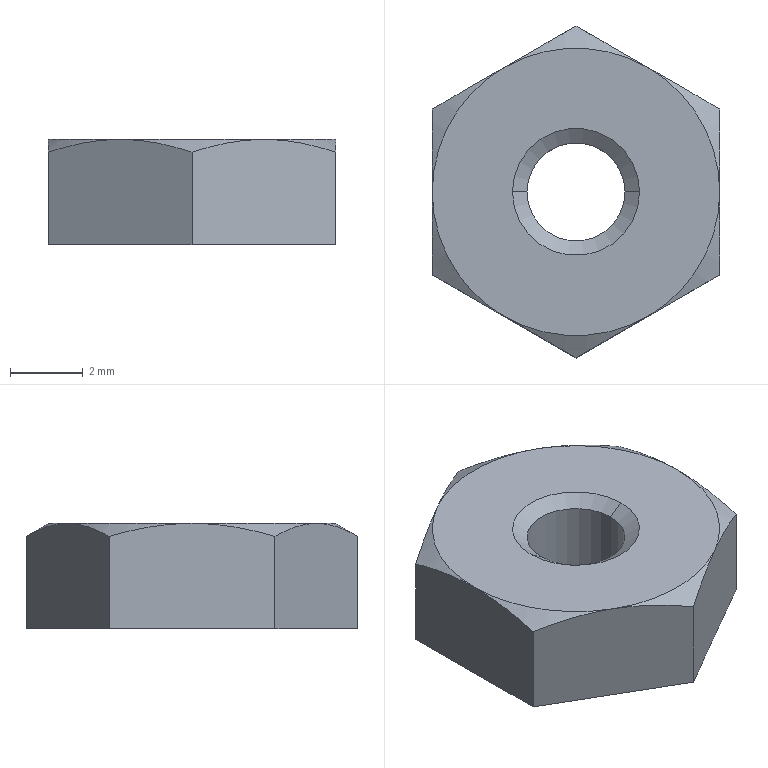Part | SolidWorks | features BaseBody 1 | 1 solid | 22 faces | box 7.925 x 9.151 x 2.896 mm | volume 139.153 mm3 | cone 10 | plane 8 | cylinder 4 | commonest cylinder face diameters 2.705 x2 3.505 x2
STEP:
#1=CARTESIAN_POINT('',(1.753,0.,-2.896));
#2=VERTEX_POINT('',#1);
#3=CARTESIAN_POINT('',(-1.753,0.,-2.896));
#4=VERTEX_POINT('',#3);
#5=CARTESIAN_POINT('',(0.,0.,-2.896));
#6=DIRECTION('',(0.,0.,-1.));
#7=DIRECTION('',(1.,0.,0.));
#8=AXIS2_PLACEMENT_3D('',#5,#6,#7);
#9=CIRCLE('',#8,1.753);
#10=EDGE_CURVE('',#2,#4,#9,.T.);
#11=ORIENTED_EDGE('',*,*,#10,.T.);
#12=CARTESIAN_POINT('',(-1.753,0.,-2.87));
#13=VERTEX_POINT('',#12);
#14=CARTESIAN_POINT('',(-1.753,0.,-2.896));
#15=DIRECTION('',(0.,0.,1.));
#16=VECTOR('',#15,1000.);
#17=LINE('',#14,#16);
#18=EDGE_CURVE('',#4,#13,#17,.T.);
#19=ORIENTED_EDGE('',*,*,#18,.T.);
#20=CARTESIAN_POINT('',(1.753,0.,-2.87));
#21=VERTEX_POINT('',#20);
#22=CARTESIAN_POINT('',(0.,0.,-2.87));
#23=DIRECTION('',(0.,0.,1.));
#24=DIRECTION('',(1.,0.,0.));
#25=AXIS2_PLACEMENT_3D('',#22,#23,#24);
#26=CIRCLE('',#25,1.753);
#27=EDGE_CURVE('',#13,#21,#26,.T.);
#28=ORIENTED_EDGE('',*,*,#27,.T.);
#29=CARTESIAN_POINT('',(1.753,0.,-2.896));
#30=DIRECTION('',(0.,0.,1.));
#31=VECTOR('',#30,1000.);
#32=LINE('',#29,#31);
#33=EDGE_CURVE('',#2,#21,#32,.T.);
#34=ORIENTED_EDGE('',*,*,#33,.F.);
#35=EDGE_LOOP('',(#11,#19,#28,#34));
#36=FACE_OUTER_BOUND('',#35,.T.);
#37=CARTESIAN_POINT('',(0.,0.,-2.896));
#38=DIRECTION('',(0.,0.,1.));
#39=DIRECTION('',(1.,0.,0.));
#40=AXIS2_PLACEMENT_3D('',#37,#38,#39);
#41=CYLINDRICAL_SURFACE('',#40,1.753);
#42=ADVANCED_FACE('',(#36),#41,.F.);
#43=CARTESIAN_POINT('',(-1.353,0.,-2.59));
#44=VERTEX_POINT('',#43);
#45=CARTESIAN_POINT('',(1.353,0.,-2.59));
#46=VERTEX_POINT('',#45);
#47=CARTESIAN_POINT('',(0.,0.,-2.59));
#48=DIRECTION('',(0.,0.,1.));
#49=DIRECTION('',(-1.,0.,0.));
#50=AXIS2_PLACEMENT_3D('',#47,#48,#49);
#51=CIRCLE('',#50,1.353);
#52=EDGE_CURVE('',#44,#46,#51,.T.);
#53=ORIENTED_EDGE('',*,*,#52,.T.);
#54=CARTESIAN_POINT('',(1.353,0.,-2.59));
#55=DIRECTION('',(0.8192,0.,-0.5736));
#56=VECTOR('',#55,1000.);
#57=LINE('',#54,#56);
#58=EDGE_CURVE('',#46,#21,#57,.T.);
#59=ORIENTED_EDGE('',*,*,#58,.T.);
#60=ORIENTED_EDGE('',*,*,#27,.F.);
#61=CARTESIAN_POINT('',(-1.353,0.,-2.59));
#62=DIRECTION('',(-0.8192,0.,-0.5736));
#63=VECTOR('',#62,1000.);
#64=LINE('',#61,#63);
#65=EDGE_CURVE('',#44,#13,#64,.T.);
#66=ORIENTED_EDGE('',*,*,#65,.F.);
#67=EDGE_LOOP('',(#53,#59,#60,#66));
#68=FACE_OUTER_BOUND('',#67,.T.);
#69=CARTESIAN_POINT('',(0.,0.,-2.59));
#70=DIRECTION('',(0.,0.,-1.));
#71=DIRECTION('',(-1.,0.,0.));
#72=AXIS2_PLACEMENT_3D('',#69,#70,#71);
#73=CONICAL_SURFACE('',#72,1.353,0.9599);
#74=ADVANCED_FACE('',(#68),#73,.F.);
#75=ORIENTED_EDGE('',*,*,#52,.F.);
#76=CARTESIAN_POINT('',(-1.353,0.,-0.2801));
#77=VERTEX_POINT('',#76);
#78=CARTESIAN_POINT('',(-1.353,0.,-2.59));
#79=DIRECTION('',(0.,0.,1.));
#80=VECTOR('',#79,1000.);
#81=LINE('',#78,#80);
#82=EDGE_CURVE('',#44,#77,#81,.T.);
#83=ORIENTED_EDGE('',*,*,#82,.T.);
#84=CARTESIAN_POINT('',(1.353,0.,-0.2801));
#85=VERTEX_POINT('',#84);
#86=CARTESIAN_POINT('',(0.,0.,-0.2801));
#87=DIRECTION('',(0.,0.,1.));
#88=DIRECTION('',(1.,0.,0.));
#89=AXIS2_PLACEMENT_3D('',#86,#87,#88);
#90=CIRCLE('',#89,1.353);
#91=EDGE_CURVE('',#77,#85,#90,.T.);
#92=ORIENTED_EDGE('',*,*,#91,.T.);
#93=CARTESIAN_POINT('',(1.353,0.,-2.59));
#94=DIRECTION('',(0.,0.,1.));
#95=VECTOR('',#94,1000.);
#96=LINE('',#93,#95);
#97=EDGE_CURVE('',#46,#85,#96,.T.);
#98=ORIENTED_EDGE('',*,*,#97,.F.);
#99=EDGE_LOOP('',(#75,#83,#92,#98));
#100=FACE_OUTER_BOUND('',#99,.T.);
#101=CARTESIAN_POINT('',(0.,0.,-2.59));
#102=DIRECTION('',(0.,0.,1.));
#103=DIRECTION('',(1.,0.,0.));
#104=AXIS2_PLACEMENT_3D('',#101,#102,#103);
#105=CYLINDRICAL_SURFACE('',#104,1.353);
#106=ADVANCED_FACE('',(#100),#105,.F.);
#107=ORIENTED_EDGE('',*,*,#91,.F.);
#108=CARTESIAN_POINT('',(-1.753,0.,0.));
#109=VERTEX_POINT('',#108);
#110=CARTESIAN_POINT('',(-1.353,0.,-0.2801));
#111=DIRECTION('',(-0.8192,0.,0.5736));
#112=VECTOR('',#111,1000.);
#113=LINE('',#110,#112);
#114=EDGE_CURVE('',#77,#109,#113,.T.);
#115=ORIENTED_EDGE('',*,*,#114,.T.);
#116=CARTESIAN_POINT('',(1.753,0.,0.));
#117=VERTEX_POINT('',#116);
#118=CARTESIAN_POINT('',(0.,0.,0.));
#119=DIRECTION('',(0.,0.,1.));
#120=DIRECTION('',(1.,0.,0.));
#121=AXIS2_PLACEMENT_3D('',#118,#119,#120);
#122=CIRCLE('',#121,1.753);
#123=EDGE_CURVE('',#109,#117,#122,.T.);
#124=ORIENTED_EDGE('',*,*,#123,.T.);
#125=CARTESIAN_POINT('',(1.353,0.,-0.2801));
#126=DIRECTION('',(0.8192,0.,0.5736));
#127=VECTOR('',#126,1000.);
#128=LINE('',#125,#127);
#129=EDGE_CURVE('',#85,#117,#128,.T.);
#130=ORIENTED_EDGE('',*,*,#129,.F.);
#131=EDGE_LOOP('',(#107,#115,#124,#130));
#132=FACE_OUTER_BOUND('',#131,.T.);
#133=CARTESIAN_POINT('',(0.,0.,-0.2801));
#134=DIRECTION('',(0.,0.,1.));
#135=DIRECTION('',(1.,0.,0.));
#136=AXIS2_PLACEMENT_3D('',#133,#134,#135);
#137=CONICAL_SURFACE('',#136,1.353,0.9599);
#138=ADVANCED_FACE('',(#132),#137,.F.);
#139=ORIENTED_EDGE('',*,*,#18,.F.);
#140=CARTESIAN_POINT('',(0.,0.,-2.896));
#141=DIRECTION('',(0.,0.,-1.));
#142=DIRECTION('',(1.,0.,0.));
#143=AXIS2_PLACEMENT_3D('',#140,#141,#142);
#144=CIRCLE('',#143,1.753);
#145=EDGE_CURVE('',#4,#2,#144,.T.);
#146=ORIENTED_EDGE('',*,*,#145,.T.);
#147=ORIENTED_EDGE('',*,*,#33,.T.);
#148=CARTESIAN_POINT('',(0.,0.,-2.87));
#149=DIRECTION('',(0.,0.,1.));
#150=DIRECTION('',(1.,0.,0.));
#151=AXIS2_PLACEMENT_3D('',#148,#149,#150);
#152=CIRCLE('',#151,1.753);
#153=EDGE_CURVE('',#21,#13,#152,.T.);
#154=ORIENTED_EDGE('',*,*,#153,.T.);
#155=EDGE_LOOP('',(#139,#146,#147,#154));
#156=FACE_OUTER_BOUND('',#155,.T.);
#157=CARTESIAN_POINT('',(0.,0.,-2.896));
#158=DIRECTION('',(0.,0.,1.));
#159=DIRECTION('',(1.,0.,0.));
#160=AXIS2_PLACEMENT_3D('',#157,#158,#159);
#161=CYLINDRICAL_SURFACE('',#160,1.753);
#162=ADVANCED_FACE('',(#156),#161,.F.);
#163=ORIENTED_EDGE('',*,*,#58,.F.);
#164=CARTESIAN_POINT('',(0.,0.,-2.59));
#165=DIRECTION('',(0.,0.,1.));
#166=DIRECTION('',(-1.,0.,0.));
#167=AXIS2_PLACEMENT_3D('',#164,#165,#166);
#168=CIRCLE('',#167,1.353);
#169=EDGE_CURVE('',#46,#44,#168,.T.);
#170=ORIENTED_EDGE('',*,*,#169,.T.);
#171=ORIENTED_EDGE('',*,*,#65,.T.);
#172=ORIENTED_EDGE('',*,*,#153,.F.);
#173=EDGE_LOOP('',(#163,#170,#171,#172));
#174=FACE_OUTER_BOUND('',#173,.T.);
#175=CARTESIAN_POINT('',(0.,0.,-2.59));
#176=DIRECTION('',(0.,0.,-1.));
#177=DIRECTION('',(-1.,0.,0.));
#178=AXIS2_PLACEMENT_3D('',#175,#176,#177);
#179=CONICAL_SURFACE('',#178,1.353,0.9599);
#180=ADVANCED_FACE('',(#174),#179,.F.);
#181=ORIENTED_EDGE('',*,*,#10,.F.);
#182=ORIENTED_EDGE('',*,*,#145,.F.);
#183=EDGE_LOOP('',(#181,#182));
#184=FACE_BOUND('',#183,.T.);
#185=CARTESIAN_POINT('',(0.,-4.575,-2.896));
#186=VERTEX_POINT('',#185);
#187=CARTESIAN_POINT('',(-3.962,-2.288,-2.896));
#188=VERTEX_POINT('',#187);
#189=CARTESIAN_POINT('',(0.,-4.575,-2.896));
#190=DIRECTION('',(-0.866,0.5,0.));
#191=VECTOR('',#190,1000.);
#192=LINE('',#189,#191);
#193=EDGE_CURVE('',#186,#188,#192,.T.);
#194=ORIENTED_EDGE('',*,*,#193,.T.);
#195=CARTESIAN_POINT('',(-3.962,2.288,-2.896));
#196=VERTEX_POINT('',#195);
#197=CARTESIAN_POINT('',(-3.962,0.,-2.896));
#198=DIRECTION('',(0.,1.,0.));
#199=VECTOR('',#198,1000.);
#200=LINE('',#197,#199);
#201=EDGE_CURVE('',#188,#196,#200,.T.);
#202=ORIENTED_EDGE('',*,*,#201,.T.);
#203=CARTESIAN_POINT('',(0.,4.575,-2.896));
#204=VERTEX_POINT('',#203);
#205=CARTESIAN_POINT('',(-3.962,2.288,-2.896));
#206=DIRECTION('',(0.866,0.5,0.));
#207=VECTOR('',#206,1000.);
#208=LINE('',#205,#207);
#209=EDGE_CURVE('',#196,#204,#208,.T.);
#210=ORIENTED_EDGE('',*,*,#209,.T.);
#211=CARTESIAN_POINT('',(3.962,2.288,-2.896));
#212=VERTEX_POINT('',#211);
#213=CARTESIAN_POINT('',(0.,4.575,-2.896));
#214=DIRECTION('',(0.866,-0.5,0.));
#215=VECTOR('',#214,1000.);
#216=LINE('',#213,#215);
#217=EDGE_CURVE('',#204,#212,#216,.T.);
#218=ORIENTED_EDGE('',*,*,#217,.T.);
#219=CARTESIAN_POINT('',(3.962,-2.288,-2.896));
#220=VERTEX_POINT('',#219);
#221=CARTESIAN_POINT('',(3.962,0.,-2.896));
#222=DIRECTION('',(0.,-1.,0.));
#223=VECTOR('',#222,1000.);
#224=LINE('',#221,#223);
#225=EDGE_CURVE('',#212,#220,#224,.T.);
#226=ORIENTED_EDGE('',*,*,#225,.T.);
#227=CARTESIAN_POINT('',(3.962,-2.288,-2.896));
#228=DIRECTION('',(-0.866,-0.5,0.));
#229=VECTOR('',#228,1000.);
#230=LINE('',#227,#229);
#231=EDGE_CURVE('',#220,#186,#230,.T.);
#232=ORIENTED_EDGE('',*,*,#231,.T.);
#233=EDGE_LOOP('',(#194,#202,#210,#218,#226,#232));
#234=FACE_OUTER_BOUND('',#233,.T.);
#235=CARTESIAN_POINT('',(3.962,-4.63,-2.896));
#236=DIRECTION('',(0.,0.,-1.));
#237=DIRECTION('',(-1.,0.,0.));
#238=AXIS2_PLACEMENT_3D('',#235,#236,#237);
#239=PLANE('',#238);
#240=ADVANCED_FACE('',(#184,#234),#239,.T.);
#241=ORIENTED_EDGE('',*,*,#82,.F.);
#242=ORIENTED_EDGE('',*,*,#169,.F.);
#243=ORIENTED_EDGE('',*,*,#97,.T.);
#244=CARTESIAN_POINT('',(0.,0.,-0.2801));
#245=DIRECTION('',(0.,0.,1.));
#246=DIRECTION('',(1.,0.,0.));
#247=AXIS2_PLACEMENT_3D('',#244,#245,#246);
#248=CIRCLE('',#247,1.353);
#249=EDGE_CURVE('',#85,#77,#248,.T.);
#250=ORIENTED_EDGE('',*,*,#249,.T.);
#251=EDGE_LOOP('',(#241,#242,#243,#250));
#252=FACE_OUTER_BOUND('',#251,.T.);
#253=CARTESIAN_POINT('',(0.,0.,-2.59));
#254=DIRECTION('',(0.,0.,1.));
#255=DIRECTION('',(1.,0.,0.));
#256=AXIS2_PLACEMENT_3D('',#253,#254,#255);
#257=CYLINDRICAL_SURFACE('',#256,1.353);
#258=ADVANCED_FACE('',(#252),#257,.F.);
#259=CARTESIAN_POINT('',(-3.962,2.288,-0.3539));
#260=VERTEX_POINT('',#259);
#261=CARTESIAN_POINT('',(-3.962,2.288,-1.439));
#262=DIRECTION('',(0.,0.,-1.));
#263=VECTOR('',#262,1000.);
#264=LINE('',#261,#263);
#265=EDGE_CURVE('',#260,#196,#264,.T.);
#266=ORIENTED_EDGE('',*,*,#265,.T.);
#267=ORIENTED_EDGE('',*,*,#201,.F.);
#268=CARTESIAN_POINT('',(-3.962,-2.288,-0.3539));
#269=VERTEX_POINT('',#268);
#270=CARTESIAN_POINT('',(-3.962,-2.288,-1.439));
#271=DIRECTION('',(0.,0.,1.));
#272=VECTOR('',#271,1000.);
#273=LINE('',#270,#272);
#274=EDGE_CURVE('',#188,#269,#273,.T.);
#275=ORIENTED_EDGE('',*,*,#274,.T.);
#276=CARTESIAN_POINT('',(-3.962,0.,0.));
#277=VERTEX_POINT('',#276);
#278=CARTESIAN_POINT('',(-3.962,-2.288,-0.3539));
#279=CARTESIAN_POINT('',(-3.962,-1.54,-0.1381));
#280=CARTESIAN_POINT('',(-3.962,-0.7808,0.));
#281=CARTESIAN_POINT('',(-3.962,0.,0.));
#282=B_SPLINE_CURVE_WITH_KNOTS('',3,(#278,#279,#280,#281),.UNSPECIFIED.,.F.,.F.,(4,4),(0.,0.002315),.UNSPECIFIED.);
#283=EDGE_CURVE('',#269,#277,#282,.T.);
#284=ORIENTED_EDGE('',*,*,#283,.T.);
#285=CARTESIAN_POINT('',(-3.962,0.,0.));
#286=CARTESIAN_POINT('',(-3.962,0.7808,0.));
#287=CARTESIAN_POINT('',(-3.962,1.54,-0.1381));
#288=CARTESIAN_POINT('',(-3.962,2.288,-0.3539));
#289=B_SPLINE_CURVE_WITH_KNOTS('',3,(#285,#286,#287,#288),.UNSPECIFIED.,.F.,.F.,(4,4),(0.,0.002315),.UNSPECIFIED.);
#290=EDGE_CURVE('',#277,#260,#289,.T.);
#291=ORIENTED_EDGE('',*,*,#290,.T.);
#292=EDGE_LOOP('',(#266,#267,#275,#284,#291));
#293=FACE_OUTER_BOUND('',#292,.T.);
#294=CARTESIAN_POINT('',(-3.962,-2.288,-2.896));
#295=DIRECTION('',(-1.,0.,0.));
#296=DIRECTION('',(0.,0.,1.));
#297=AXIS2_PLACEMENT_3D('',#294,#295,#296);
#298=PLANE('',#297);
#299=ADVANCED_FACE('',(#293),#298,.T.);
#300=ORIENTED_EDGE('',*,*,#274,.F.);
#301=ORIENTED_EDGE('',*,*,#193,.F.);
#302=CARTESIAN_POINT('',(0.,-4.575,-0.3539));
#303=VERTEX_POINT('',#302);
#304=CARTESIAN_POINT('',(0.,-4.575,-1.439));
#305=DIRECTION('',(0.,0.,1.));
#306=VECTOR('',#305,1000.);
#307=LINE('',#304,#306);
#308=EDGE_CURVE('',#186,#303,#307,.T.);
#309=ORIENTED_EDGE('',*,*,#308,.T.);
#310=CARTESIAN_POINT('',(-1.981,-3.432,0.));
#311=VERTEX_POINT('',#310);
#312=CARTESIAN_POINT('',(0.,-4.575,-0.3539));
#313=CARTESIAN_POINT('',(-0.6473,-4.202,-0.1381));
#314=CARTESIAN_POINT('',(-1.305,-3.822,0.));
#315=CARTESIAN_POINT('',(-1.981,-3.432,0.));
#316=B_SPLINE_CURVE_WITH_KNOTS('',3,(#312,#313,#314,#315),.UNSPECIFIED.,.F.,.F.,(4,4),(0.,0.002315),.UNSPECIFIED.);
#317=EDGE_CURVE('',#303,#311,#316,.T.);
#318=ORIENTED_EDGE('',*,*,#317,.T.);
#319=CARTESIAN_POINT('',(-1.981,-3.432,0.));
#320=CARTESIAN_POINT('',(-2.657,-3.041,0.));
#321=CARTESIAN_POINT('',(-3.315,-2.661,-0.1381));
#322=CARTESIAN_POINT('',(-3.962,-2.288,-0.3539));
#323=B_SPLINE_CURVE_WITH_KNOTS('',3,(#319,#320,#321,#322),.UNSPECIFIED.,.F.,.F.,(4,4),(0.,0.002315),.UNSPECIFIED.);
#324=EDGE_CURVE('',#311,#269,#323,.T.);
#325=ORIENTED_EDGE('',*,*,#324,.T.);
#326=EDGE_LOOP('',(#300,#301,#309,#318,#325));
#327=FACE_OUTER_BOUND('',#326,.T.);
#328=CARTESIAN_POINT('',(-3.962,-2.288,-2.896));
#329=DIRECTION('',(-0.5,-0.866,0.));
#330=DIRECTION('',(0.866,-0.5,0.));
#331=AXIS2_PLACEMENT_3D('',#328,#329,#330);
#332=PLANE('',#331);
#333=ADVANCED_FACE('',(#327),#332,.T.);
#334=ORIENTED_EDGE('',*,*,#308,.F.);
#335=ORIENTED_EDGE('',*,*,#231,.F.);
#336=CARTESIAN_POINT('',(3.962,-2.288,-0.3539));
#337=VERTEX_POINT('',#336);
#338=CARTESIAN_POINT('',(3.962,-2.288,-1.439));
#339=DIRECTION('',(0.,0.,1.));
#340=VECTOR('',#339,1000.);
#341=LINE('',#338,#340);
#342=EDGE_CURVE('',#220,#337,#341,.T.);
#343=ORIENTED_EDGE('',*,*,#342,.T.);
#344=CARTESIAN_POINT('',(1.981,-3.432,0.));
#345=VERTEX_POINT('',#344);
#346=CARTESIAN_POINT('',(3.962,-2.288,-0.3539));
#347=CARTESIAN_POINT('',(3.315,-2.661,-0.1381));
#348=CARTESIAN_POINT('',(2.657,-3.041,0.));
#349=CARTESIAN_POINT('',(1.981,-3.432,0.));
#350=B_SPLINE_CURVE_WITH_KNOTS('',3,(#346,#347,#348,#349),.UNSPECIFIED.,.F.,.F.,(4,4),(0.,0.002315),.UNSPECIFIED.);
#351=EDGE_CURVE('',#337,#345,#350,.T.);
#352=ORIENTED_EDGE('',*,*,#351,.T.);
#353=CARTESIAN_POINT('',(1.981,-3.432,0.));
#354=CARTESIAN_POINT('',(1.305,-3.822,0.));
#355=CARTESIAN_POINT('',(0.6473,-4.202,-0.1381));
#356=CARTESIAN_POINT('',(0.,-4.575,-0.3539));
#357=B_SPLINE_CURVE_WITH_KNOTS('',3,(#353,#354,#355,#356),.UNSPECIFIED.,.F.,.F.,(4,4),(0.,0.002315),.UNSPECIFIED.);
#358=EDGE_CURVE('',#345,#303,#357,.T.);
#359=ORIENTED_EDGE('',*,*,#358,.T.);
#360=EDGE_LOOP('',(#334,#335,#343,#352,#359));
#361=FACE_OUTER_BOUND('',#360,.T.);
#362=CARTESIAN_POINT('',(0.,-4.575,-2.896));
#363=DIRECTION('',(0.5,-0.866,0.));
#364=DIRECTION('',(0.866,0.5,0.));
#365=AXIS2_PLACEMENT_3D('',#362,#363,#364);
#366=PLANE('',#365);
#367=ADVANCED_FACE('',(#361),#366,.T.);
#368=ORIENTED_EDGE('',*,*,#342,.F.);
#369=ORIENTED_EDGE('',*,*,#225,.F.);
#370=CARTESIAN_POINT('',(3.962,2.288,-0.3539));
#371=VERTEX_POINT('',#370);
#372=CARTESIAN_POINT('',(3.962,2.288,-1.439));
#373=DIRECTION('',(0.,0.,-1.));
#374=VECTOR('',#373,1000.);
#375=LINE('',#372,#374);
#376=EDGE_CURVE('',#371,#212,#375,.T.);
#377=ORIENTED_EDGE('',*,*,#376,.F.);
#378=CARTESIAN_POINT('',(3.962,-0.000000001,0.));
#379=VERTEX_POINT('',#378);
#380=CARTESIAN_POINT('',(3.962,-0.000000001,0.));
#381=CARTESIAN_POINT('',(3.962,0.7808,0.));
#382=CARTESIAN_POINT('',(3.962,1.54,-0.1381));
#383=CARTESIAN_POINT('',(3.962,2.288,-0.3539));
#384=B_SPLINE_CURVE_WITH_KNOTS('',3,(#380,#381,#382,#383),.UNSPECIFIED.,.F.,.F.,(4,4),(0.,0.002315),.UNSPECIFIED.);
#385=EDGE_CURVE('',#379,#371,#384,.T.);
#386=ORIENTED_EDGE('',*,*,#385,.F.);
#387=CARTESIAN_POINT('',(3.962,-2.288,-0.3539));
#388=CARTESIAN_POINT('',(3.962,-1.54,-0.1381));
#389=CARTESIAN_POINT('',(3.962,-0.7808,0.));
#390=CARTESIAN_POINT('',(3.962,-0.000000001,0.));
#391=B_SPLINE_CURVE_WITH_KNOTS('',3,(#387,#388,#389,#390),.UNSPECIFIED.,.F.,.F.,(4,4),(0.,0.002315),.UNSPECIFIED.);
#392=EDGE_CURVE('',#337,#379,#391,.T.);
#393=ORIENTED_EDGE('',*,*,#392,.F.);
#394=EDGE_LOOP('',(#368,#369,#377,#386,#393));
#395=FACE_OUTER_BOUND('',#394,.T.);
#396=CARTESIAN_POINT('',(3.962,-2.288,-2.896));
#397=DIRECTION('',(-1.,0.,0.));
#398=DIRECTION('',(0.,0.,1.));
#399=AXIS2_PLACEMENT_3D('',#396,#397,#398);
#400=PLANE('',#399);
#401=ADVANCED_FACE('',(#395),#400,.F.);
#402=ORIENTED_EDGE('',*,*,#376,.T.);
#403=ORIENTED_EDGE('',*,*,#217,.F.);
#404=CARTESIAN_POINT('',(0.,4.575,-0.3539));
#405=VERTEX_POINT('',#404);
#406=CARTESIAN_POINT('',(0.,4.575,-1.439));
#407=DIRECTION('',(0.,0.,1.));
#408=VECTOR('',#407,1000.);
#409=LINE('',#406,#408);
#410=EDGE_CURVE('',#204,#405,#409,.T.);
#411=ORIENTED_EDGE('',*,*,#410,.T.);
#412=CARTESIAN_POINT('',(1.981,3.432,0.));
#413=VERTEX_POINT('',#412);
#414=CARTESIAN_POINT('',(0.,4.575,-0.3539));
#415=CARTESIAN_POINT('',(0.6473,4.202,-0.1381));
#416=CARTESIAN_POINT('',(1.305,3.822,0.));
#417=CARTESIAN_POINT('',(1.981,3.432,0.));
#418=B_SPLINE_CURVE_WITH_KNOTS('',3,(#414,#415,#416,#417),.UNSPECIFIED.,.F.,.F.,(4,4),(0.,0.002315),.UNSPECIFIED.);
#419=EDGE_CURVE('',#405,#413,#418,.T.);
#420=ORIENTED_EDGE('',*,*,#419,.T.);
#421=CARTESIAN_POINT('',(1.981,3.432,0.));
#422=CARTESIAN_POINT('',(2.657,3.041,0.));
#423=CARTESIAN_POINT('',(3.315,2.661,-0.1381));
#424=CARTESIAN_POINT('',(3.962,2.288,-0.3539));
#425=B_SPLINE_CURVE_WITH_KNOTS('',3,(#421,#422,#423,#424),.UNSPECIFIED.,.F.,.F.,(4,4),(0.,0.002315),.UNSPECIFIED.);
#426=EDGE_CURVE('',#413,#371,#425,.T.);
#427=ORIENTED_EDGE('',*,*,#426,.T.);
#428=EDGE_LOOP('',(#402,#403,#411,#420,#427));
#429=FACE_OUTER_BOUND('',#428,.T.);
#430=CARTESIAN_POINT('',(3.962,2.288,-2.896));
#431=DIRECTION('',(0.5,0.866,0.));
#432=DIRECTION('',(-0.866,0.5,0.));
#433=AXIS2_PLACEMENT_3D('',#430,#431,#432);
#434=PLANE('',#433);
#435=ADVANCED_FACE('',(#429),#434,.T.);
#436=ORIENTED_EDGE('',*,*,#410,.F.);
#437=ORIENTED_EDGE('',*,*,#209,.F.);
#438=ORIENTED_EDGE('',*,*,#265,.F.);
#439=CARTESIAN_POINT('',(-1.981,3.432,0.));
#440=VERTEX_POINT('',#439);
#441=CARTESIAN_POINT('',(-3.962,2.288,-0.3539));
#442=CARTESIAN_POINT('',(-3.315,2.661,-0.1381));
#443=CARTESIAN_POINT('',(-2.657,3.041,0.));
#444=CARTESIAN_POINT('',(-1.981,3.432,0.));
#445=B_SPLINE_CURVE_WITH_KNOTS('',3,(#441,#442,#443,#444),.UNSPECIFIED.,.F.,.F.,(4,4),(0.,0.002315),.UNSPECIFIED.);
#446=EDGE_CURVE('',#260,#440,#445,.T.);
#447=ORIENTED_EDGE('',*,*,#446,.T.);
#448=CARTESIAN_POINT('',(-1.981,3.432,0.));
#449=CARTESIAN_POINT('',(-1.305,3.822,0.));
#450=CARTESIAN_POINT('',(-0.6473,4.202,-0.1381));
#451=CARTESIAN_POINT('',(0.,4.575,-0.3539));
#452=B_SPLINE_CURVE_WITH_KNOTS('',3,(#448,#449,#450,#451),.UNSPECIFIED.,.F.,.F.,(4,4),(0.,0.002315),.UNSPECIFIED.);
#453=EDGE_CURVE('',#440,#405,#452,.T.);
#454=ORIENTED_EDGE('',*,*,#453,.T.);
#455=EDGE_LOOP('',(#436,#437,#438,#447,#454));
#456=FACE_OUTER_BOUND('',#455,.T.);
#457=CARTESIAN_POINT('',(0.,4.575,-2.896));
#458=DIRECTION('',(-0.5,0.866,0.));
#459=DIRECTION('',(-0.866,-0.5,0.));
#460=AXIS2_PLACEMENT_3D('',#457,#458,#459);
#461=PLANE('',#460);
#462=ADVANCED_FACE('',(#456),#461,.T.);
#463=ORIENTED_EDGE('',*,*,#114,.F.);
#464=ORIENTED_EDGE('',*,*,#249,.F.);
#465=ORIENTED_EDGE('',*,*,#129,.T.);
#466=CARTESIAN_POINT('',(0.,0.,0.));
#467=DIRECTION('',(0.,0.,1.));
#468=DIRECTION('',(1.,0.,0.));
#469=AXIS2_PLACEMENT_3D('',#466,#467,#468);
#470=CIRCLE('',#469,1.753);
#471=EDGE_CURVE('',#117,#109,#470,.T.);
#472=ORIENTED_EDGE('',*,*,#471,.T.);
#473=EDGE_LOOP('',(#463,#464,#465,#472));
#474=FACE_OUTER_BOUND('',#473,.T.);
#475=CARTESIAN_POINT('',(0.,0.,-0.2801));
#476=DIRECTION('',(0.,0.,1.));
#477=DIRECTION('',(1.,0.,0.));
#478=AXIS2_PLACEMENT_3D('',#475,#476,#477);
#479=CONICAL_SURFACE('',#478,1.353,0.9599);
#480=ADVANCED_FACE('',(#474),#479,.F.);
#481=CARTESIAN_POINT('',(0.,0.,0.));
#482=DIRECTION('',(0.,0.,1.));
#483=DIRECTION('',(-1.,0.,0.));
#484=AXIS2_PLACEMENT_3D('',#481,#482,#483);
#485=CIRCLE('',#484,3.962);
#486=EDGE_CURVE('',#440,#277,#485,.T.);
#487=ORIENTED_EDGE('',*,*,#486,.F.);
#488=ORIENTED_EDGE('',*,*,#446,.F.);
#489=ORIENTED_EDGE('',*,*,#290,.F.);
#490=EDGE_LOOP('',(#487,#488,#489));
#491=FACE_OUTER_BOUND('',#490,.T.);
#492=CARTESIAN_POINT('',(0.,0.,0.));
#493=DIRECTION('',(0.,0.,-1.));
#494=DIRECTION('',(-1.,0.,0.));
#495=AXIS2_PLACEMENT_3D('',#492,#493,#494);
#496=CONICAL_SURFACE('',#495,3.962,1.047);
#497=ADVANCED_FACE('',(#491),#496,.T.);
#498=ORIENTED_EDGE('',*,*,#283,.F.);
#499=ORIENTED_EDGE('',*,*,#324,.F.);
#500=CARTESIAN_POINT('',(0.,0.,0.));
#501=DIRECTION('',(0.,0.,1.));
#502=DIRECTION('',(-1.,0.,0.));
#503=AXIS2_PLACEMENT_3D('',#500,#501,#502);
#504=CIRCLE('',#503,3.962);
#505=EDGE_CURVE('',#277,#311,#504,.T.);
#506=ORIENTED_EDGE('',*,*,#505,.F.);
#507=EDGE_LOOP('',(#498,#499,#506));
#508=FACE_OUTER_BOUND('',#507,.T.);
#509=CARTESIAN_POINT('',(0.,0.,0.));
#510=DIRECTION('',(0.,0.,-1.));
#511=DIRECTION('',(-1.,0.,0.));
#512=AXIS2_PLACEMENT_3D('',#509,#510,#511);
#513=CONICAL_SURFACE('',#512,3.962,1.047);
#514=ADVANCED_FACE('',(#508),#513,.T.);
#515=ORIENTED_EDGE('',*,*,#317,.F.);
#516=ORIENTED_EDGE('',*,*,#358,.F.);
#517=CARTESIAN_POINT('',(0.,0.,0.));
#518=DIRECTION('',(0.,0.,1.));
#519=DIRECTION('',(-1.,0.,0.));
#520=AXIS2_PLACEMENT_3D('',#517,#518,#519);
#521=CIRCLE('',#520,3.962);
#522=EDGE_CURVE('',#311,#345,#521,.T.);
#523=ORIENTED_EDGE('',*,*,#522,.F.);
#524=EDGE_LOOP('',(#515,#516,#523));
#525=FACE_OUTER_BOUND('',#524,.T.);
#526=CARTESIAN_POINT('',(0.,0.,0.));
#527=DIRECTION('',(0.,0.,-1.));
#528=DIRECTION('',(-1.,0.,0.));
#529=AXIS2_PLACEMENT_3D('',#526,#527,#528);
#530=CONICAL_SURFACE('',#529,3.962,1.047);
#531=ADVANCED_FACE('',(#525),#530,.T.);
#532=CARTESIAN_POINT('',(0.,0.,0.));
#533=DIRECTION('',(0.,0.,1.));
#534=DIRECTION('',(-1.,0.,0.));
#535=AXIS2_PLACEMENT_3D('',#532,#533,#534);
#536=CIRCLE('',#535,3.962);
#537=EDGE_CURVE('',#345,#379,#536,.T.);
#538=ORIENTED_EDGE('',*,*,#537,.F.);
#539=ORIENTED_EDGE('',*,*,#351,.F.);
#540=ORIENTED_EDGE('',*,*,#392,.T.);
#541=EDGE_LOOP('',(#538,#539,#540));
#542=FACE_OUTER_BOUND('',#541,.T.);
#543=CARTESIAN_POINT('',(0.,0.,0.));
#544=DIRECTION('',(0.,0.,-1.));
#545=DIRECTION('',(-1.,0.,0.));
#546=AXIS2_PLACEMENT_3D('',#543,#544,#545);
#547=CONICAL_SURFACE('',#546,3.962,1.047);
#548=ADVANCED_FACE('',(#542),#547,.T.);
#549=ORIENTED_EDGE('',*,*,#385,.T.);
#550=ORIENTED_EDGE('',*,*,#426,.F.);
#551=CARTESIAN_POINT('',(0.,0.,0.));
#552=DIRECTION('',(0.,0.,1.));
#553=DIRECTION('',(-1.,0.,0.));
#554=AXIS2_PLACEMENT_3D('',#551,#552,#553);
#555=CIRCLE('',#554,3.962);
#556=EDGE_CURVE('',#379,#413,#555,.T.);
#557=ORIENTED_EDGE('',*,*,#556,.F.);
#558=EDGE_LOOP('',(#549,#550,#557));
#559=FACE_OUTER_BOUND('',#558,.T.);
#560=CARTESIAN_POINT('',(0.,0.,0.));
#561=DIRECTION('',(0.,0.,-1.));
#562=DIRECTION('',(-1.,0.,0.));
#563=AXIS2_PLACEMENT_3D('',#560,#561,#562);
#564=CONICAL_SURFACE('',#563,3.962,1.047);
#565=ADVANCED_FACE('',(#559),#564,.T.);
#566=ORIENTED_EDGE('',*,*,#419,.F.);
#567=ORIENTED_EDGE('',*,*,#453,.F.);
#568=CARTESIAN_POINT('',(0.,0.,0.));
#569=DIRECTION('',(0.,0.,1.));
#570=DIRECTION('',(-1.,0.,0.));
#571=AXIS2_PLACEMENT_3D('',#568,#569,#570);
#572=CIRCLE('',#571,3.962);
#573=EDGE_CURVE('',#413,#440,#572,.T.);
#574=ORIENTED_EDGE('',*,*,#573,.F.);
#575=EDGE_LOOP('',(#566,#567,#574));
#576=FACE_OUTER_BOUND('',#575,.T.);
#577=CARTESIAN_POINT('',(0.,0.,0.));
#578=DIRECTION('',(0.,0.,-1.));
#579=DIRECTION('',(-1.,0.,0.));
#580=AXIS2_PLACEMENT_3D('',#577,#578,#579);
#581=CONICAL_SURFACE('',#580,3.962,1.047);
#582=ADVANCED_FACE('',(#576),#581,.T.);
#583=ORIENTED_EDGE('',*,*,#471,.F.);
#584=ORIENTED_EDGE('',*,*,#123,.F.);
#585=EDGE_LOOP('',(#583,#584));
#586=FACE_BOUND('',#585,.T.);
#587=ORIENTED_EDGE('',*,*,#505,.T.);
#588=ORIENTED_EDGE('',*,*,#522,.T.);
#589=ORIENTED_EDGE('',*,*,#537,.T.);
#590=ORIENTED_EDGE('',*,*,#556,.T.);
#591=ORIENTED_EDGE('',*,*,#573,.T.);
#592=ORIENTED_EDGE('',*,*,#486,.T.);
#593=EDGE_LOOP('',(#587,#588,#589,#590,#591,#592));
#594=FACE_OUTER_BOUND('',#593,.T.);
#595=CARTESIAN_POINT('',(4.01,-4.01,0.));
#596=DIRECTION('',(0.,0.,-1.));
#597=DIRECTION('',(-1.,0.,0.));
#598=AXIS2_PLACEMENT_3D('',#595,#596,#597);
#599=PLANE('',#598);
#600=ADVANCED_FACE('',(#586,#594),#599,.F.);
#601=CLOSED_SHELL('',(#42,#74,#106,#138,#162,#180,#240,#258,#299,#333,#367,#401,#435,#462,#480,#497,#514,#531,#548,#565,#582,#600));
#602=MANIFOLD_SOLID_BREP('',#601);
#603=CARTESIAN_POINT('',(0.,0.,0.));
#604=DIRECTION('',(0.,0.,1.));
#605=DIRECTION('',(1.,0.,0.));
#606=AXIS2_PLACEMENT_3D('',#603,#604,#605);
#607=(LENGTH_UNIT()NAMED_UNIT(*)SI_UNIT(.MILLI.,.METRE.));
#608=UNCERTAINTY_MEASURE_WITH_UNIT(LENGTH_MEASURE(0.00001),#607,'','');
#609=(NAMED_UNIT(*)PLANE_ANGLE_UNIT()SI_UNIT($,.RADIAN.));
#610=(NAMED_UNIT(*)SI_UNIT($,.STERADIAN.)SOLID_ANGLE_UNIT());
#611=(GEOMETRIC_REPRESENTATION_CONTEXT(3)GLOBAL_UNCERTAINTY_ASSIGNED_CONTEXT((#608))GLOBAL_UNIT_ASSIGNED_CONTEXT((#607,#609,#610))REPRESENTATION_CONTEXT('',''));
#612=ADVANCED_BREP_SHAPE_REPRESENTATION('',(#602,#606),#611);